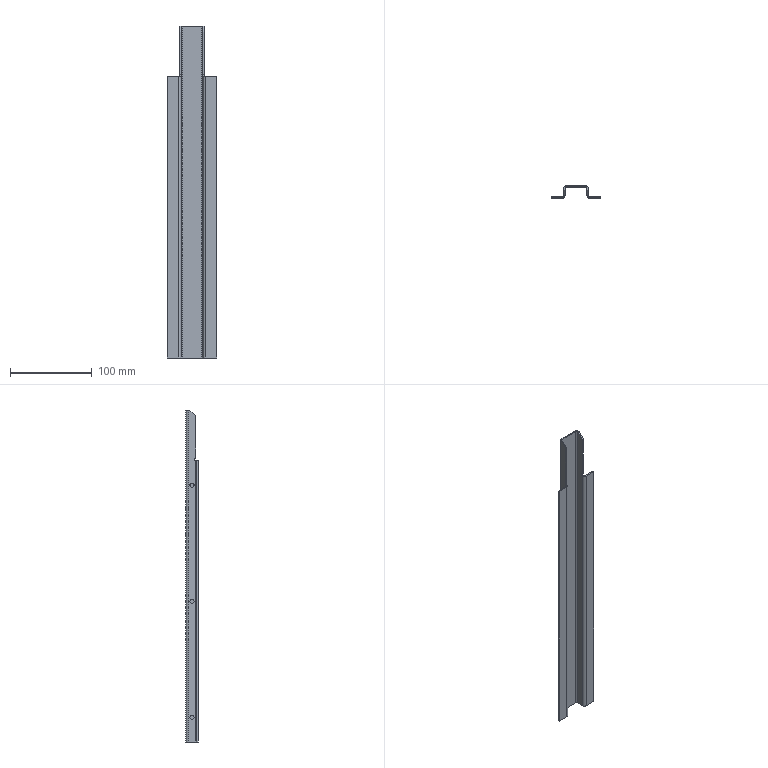Part | SolidWorks | features ICE 2, Chamfer 1, Fillet 1, FlatPattern 1, SMBaseFlange 1, SheetMetal 1 | 1 solid | 58 faces | box 60 x 15 x 406 mm | volume 50219 mm3 | plane 40 | cylinder 18 | commonest cylinder face diameters 3 x8 5 x6 6.2 x4